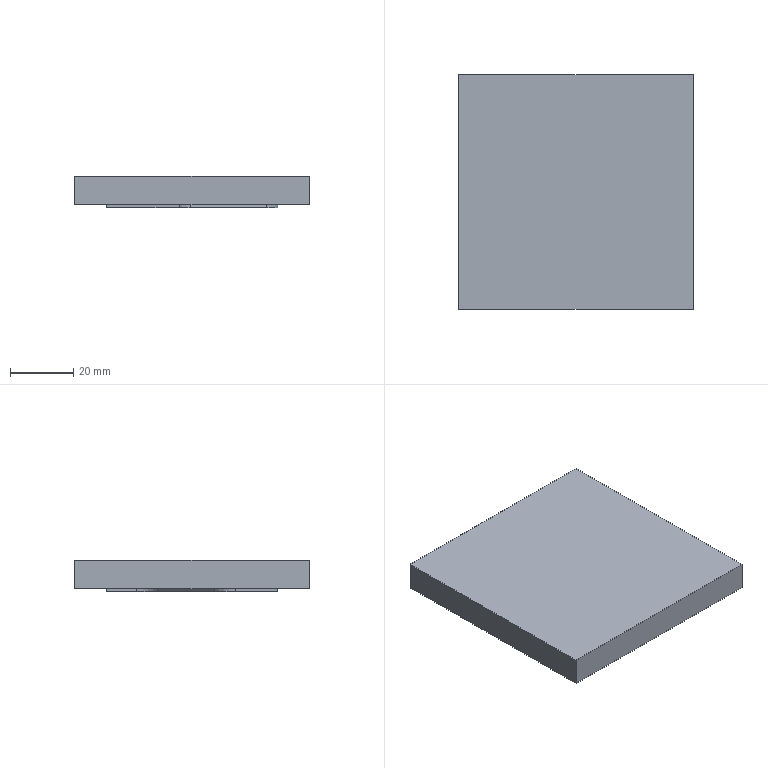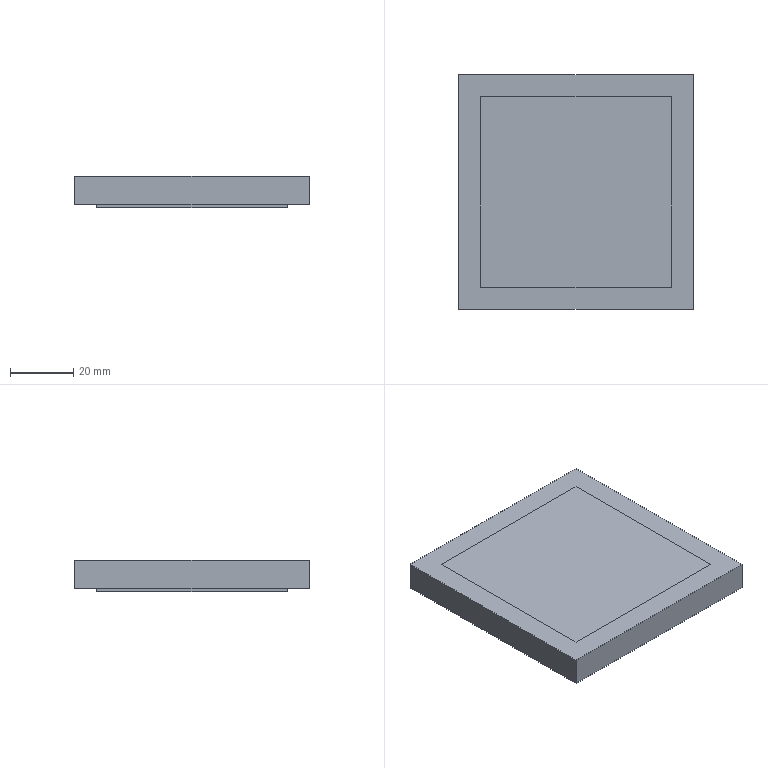CAM job | NX | 3+2 milling, drilling | part box 74 x 74 x 10 mm | stock box 74 x 74 x 10 mm
Tools:
number,name,description,diameter,corner_radius,flute_length,length,flutes
14,D10JING,Milling Tool-5 Parameters,10.0,0.0,50.0,75.0,2
1,D6A45,Milling Tool-5 Parameters,6.0,0.0,50.0,75.0,2
13,3.0ZT,Drilling Tool,3.0,0.0,35.0,50.0,2
22,2.5ZT,Drilling Tool,2.5,0.0,35.0,50.0,2
4,D10,Milling Tool-5 Parameters,10.0,0.0,50.0,75.0,2
19,D1.5,Milling Tool-5 Parameters,1.5,0.0,50.0,75.0,2
3,D63,Milling Tool-5 Parameters,63.0,0.0,50.0,75.0,2
24,9.0ZT,Drilling Tool,9.0,0.0,35.0,50.0,2
Operations:
program,operation,operation_type,tool,method,geometry_group,spindle_rpm,surface_speed,feed_per_tooth,feed_cut,feed_plunge,cut_length_mm,path_length_mm,cut_time_min,machine_time_min
1AB胶-反面见光,FLOOR_WALL_1,VolumeBased25DMillingOperation,D63,METHOD,A,6500.0,1286.0,0.1154,1500.0,100.0,286.797,340.797,0.1912,0.1966
1AB胶-反面见光,DRILLING,Operation,D6A45,METHOD,A,5000.0,94.0,0.025,250.0,0.0,28.0,239.007,0.112,0.1331
1AB胶-反面见光,DRILLING_COPY,Operation,3.0ZT,METHOD,A,2000.0,21.0,0.0375,150.0,0.0,62.408,301.252,0.4161,0.4399
1AB胶-反面见光,DRILLING_COPY_COPY,Operation,2.5ZT,METHOD,A,2000.0,21.0,0.0375,150.0,0.0,10.251,80.502,0.0683,0.0754
1AB胶-反面见光,ZLEVEL_PROFILE_1,ZLevelMilling,D10,METHOD,A,7500.0,235.0,0.2,3000.0,1000.0,1172.415,1233.815,0.4211,0.4273
1AB胶-反面见光,ZLEVEL_PROFILE_1_COPY,ZLevelMilling,D1.5,METHOD,A,7500.0,23.0,0.0533,800.0,1000.0,2178.693,2241.823,2.723,2.729
1AB胶-反面见光,ZLEVEL_PROFILE_1_COPY_COPY,ZLevelMilling,D1.5,METHOD,A,7500.0,23.0,0.0533,800.0,1000.0,463.272,526.401,0.5789,0.5852
1AB胶-反面见光,PLANAR_MILL,PlanarMilling,D6A45,METHOD,A,7500.0,141.0,0.0833,1250.0,100.0,300.115,815.705,0.2401,0.2917
2,ZLEVEL_PROFILE_1_COPY_1,ZLevelMilling,D10,METHOD,C,7500.0,235.0,0.2,3000.0,1000.0,1430.481,1483.481,0.5087,0.514
2,FLOOR_WALL_1_COPY,VolumeBased25DMillingOperation,D63,METHOD,C,6500.0,1286.0,0.1154,1500.0,100.0,1463.985,1853.174,0.976,1.015
2,PLANAR_MILL_COPY,PlanarMilling,D6A45,METHOD,C,7500.0,141.0,0.0833,1250.0,100.0,253.285,835.104,0.2026,0.2608
3,ZLEVEL_PROFILE_1_COPY_COPY_COPY,ZLevelMilling,D1.5,METHOD,B,7500.0,23.0,0.0533,800.0,1000.0,1664.273,1727.903,2.08,2.087
FIXTURE,DRILLING_COPY_1,Operation,D6A45,METHOD,D,5000.0,94.0,0.025,250.0,0.0,16.0,200.814,0.064,0.0825
FIXTURE,DRILLING_COPY_COPY_1,Operation,9.0ZT,METHOD,D,2000.0,21.0,0.0375,150.0,0.0,42.816,254.445,0.2854,0.3066
FIXTURE,ADAPTIVE_MILLING,CavityMilling,D10,METHOD,D,7500.0,235.0,0.2,3000.0,1000.0,3432.82,3490.961,1.406,1.412
FIXTURE,ZLEVEL_PROFILE_COPY,ZLevelMilling,D10JING,METHOD,D,7500.0,235.0,0.0667,1000.0,100.0,150.48,216.48,0.1505,0.1571
FIXTURE,PLANAR_MILL_COPY_COPY,PlanarMilling,D6A45,METHOD,D,7500.0,141.0,0.0833,1250.0,100.0,183.703,241.703,0.147,0.1528